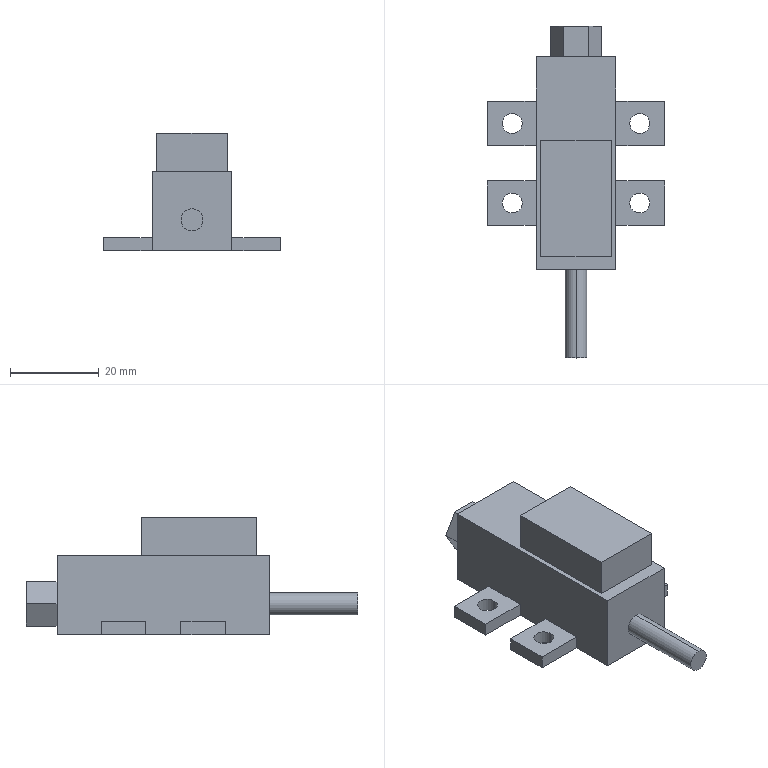Part | STEP file | NS-WY02-10 | 1 solid | 245 faces | box 40 x 75 x 26.6 mm | volume 21245 mm3 | plane 162 | spline 73 | cylinder 10 | commonest cylinder face diameters 4.5 x8 5 x2